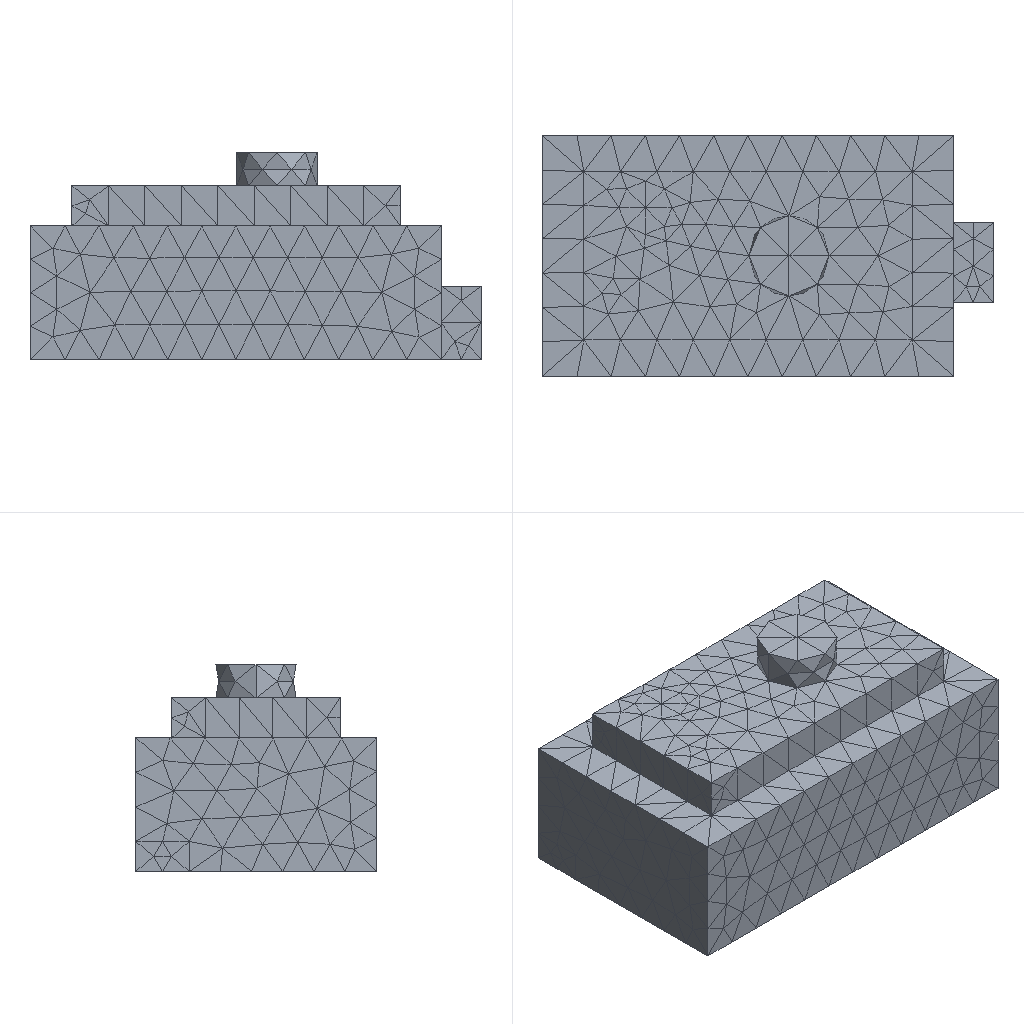Simulation study | ansys mapdl
Set-up summary:
category,name,step,type,value,unit,region
solver,ansys_mapdl
units,mm-N-s-tonne (MPa),,inferred,E=210000 density=
analysis,model,,static
mesh,nodes,,,5335
mesh,elements,,,3239
element_type,SOLID187,,,3239
material,mat 1,,E,210000
material,mat 1,,nu,0.3
load,,model,body load temp,,,all
load,,model,force,"1000 [dir=(0, 0, -1) n=402]",,node list
bc,,model,fixed,"[dofs=UX,UY,UZ n=5786]",,node list
Ansys APDL input file, long lists of numbers shortened:
/COM,ANSYS RELEASE 2026 R1           BUILD 26.1      UP20260202       09:09:40
/PREP7
/NOPR
/TITLE,2
ANTYPE, 0
*IF,_CDRDOFF,EQ,1,THEN     !if solid model was read in
_CDRDOFF=             !reset flag, numoffs already performed
*ELSE              !offset database for the following FE model
NUMOFF,NODE,     5335
NUMOFF,ELEM,     3239
NUMOFF,MAT ,        1
NUMOFF,TYPE,        1
*ENDIF
*SET,_RETURN ,  0.
*SET,_STATUS ,  0.
*SET,_UIQR   ,  402.
*SET,__FLOATPARAMETER__,  5335.
DOF,DELETE
ETBLOCK,        1,        1
(2i9,19a9)
        1      187        0        0        0        0        0        0        0        0        0        0        0        0        0        0        0        0        0        0        0
       -1
NBLOCK,6,SOLID,      5335,      5335
(3i9,6e21.13e3)
        1        0        0-4.5450000000000E+001 3.6000000000000E+001 9.0000000000000E+000
! (5334 more lines like these left out)
N,UNBL,LOC,       -1,
EBLOCK,19,SOLID,      3239,      3239
(19i10)
         1         1         1         1         0         0         0         0        10         0         1       211      1935      1936      1937      2257      2258      2259      2260
! (6477 more lines like these left out)
        -1
MPTEMP,UNBL, 1, 1,  0.    ,
MPDATA,UNBL, 1,EX  ,       1, 1,  210000.000    ,
MPTEMP,UNBL, 1, 1,  0.    ,
MPDATA,UNBL, 1,NUXY,       1, 1, 0.3    ,
MPTEMP,UNBL, 1, 1,  0.    ,
MPDATA,UNBL, 1,PRXY,       1, 1, 0.3    ,
EXTOPT,ATTR,      0,      0,      0
EXTOPT,ESIZE,  0,  0.
EXTOPT,ACLEAR,      0
TREF,  0.
IRLF,  0
BFUNIF,TEMP,_TINY
ACEL,  0.    ,  0.    ,  0.
OMEGA,  0.    ,  0.    ,  0.
DOMEGA,  0.    ,  0.    ,  0.
CGLOC,  0.    ,  0.    ,  0.
CGOMEGA,  0.    ,  0.    ,  0.
DCGOMG,  0.    ,  0.    ,  0.
KUSE,     0
TIME,  0.
ALPHAD,  0.
BETAD,  0.
DMPRAT,  0.
DMPSTR,  0.
CRPLIM, 0.1    ,   0
CRPLIM,  0.    ,   1
NCNV,     0, 1.000000000E+12,     0,  0.    ,  0.
NEQIT,     0
ERESX,DEFA
DBLOCK,      5786
(i9,a6,2(pg16.9))
        1  UX    0.00000000      0.00000000
! (5785 more lines like these left out)
       -1
FBLOCK,       402
(i9,a6,2(pg16.9))
      614  FZ   -2.48756219      0.00000000
! (401 more lines like these left out)
       -1
/GO
FINISH
Results summary:
result,analysis_type_db,,,static,unstated
result,n_sets,,,1,unstated
result,load_steps[0].set,load_step=1,,1,unstated
result,load_steps[0].substep,load_step=1,,1,unstated
result,load_steps[0].time,load_step=1,,1,unstated
result,load_steps[0].freq,load_step=1,,1,unstated
result,load_steps[0].max_usum,load_step=1,,8.74946e-05,unstated
result,load_steps[0].max_seqv,load_step=1,,0.8803,unstated
result,load_steps[0].reaction_sum.FX,load_step=1,,6.89171e-12,unstated
result,load_steps[0].reaction_sum.FY,load_step=1,,7.91975e-12,unstated
result,load_steps[0].reaction_sum.FZ,load_step=1,,1000,unstated
result,load_steps[0].reaction_sum.MX,load_step=1,,0,unstated
result,load_steps[0].reaction_sum.MY,load_step=1,,0,unstated
result,load_steps[0].reaction_sum.MZ,load_step=1,,0,unstated
result,convergence,,,results present for all listed sets,unstated